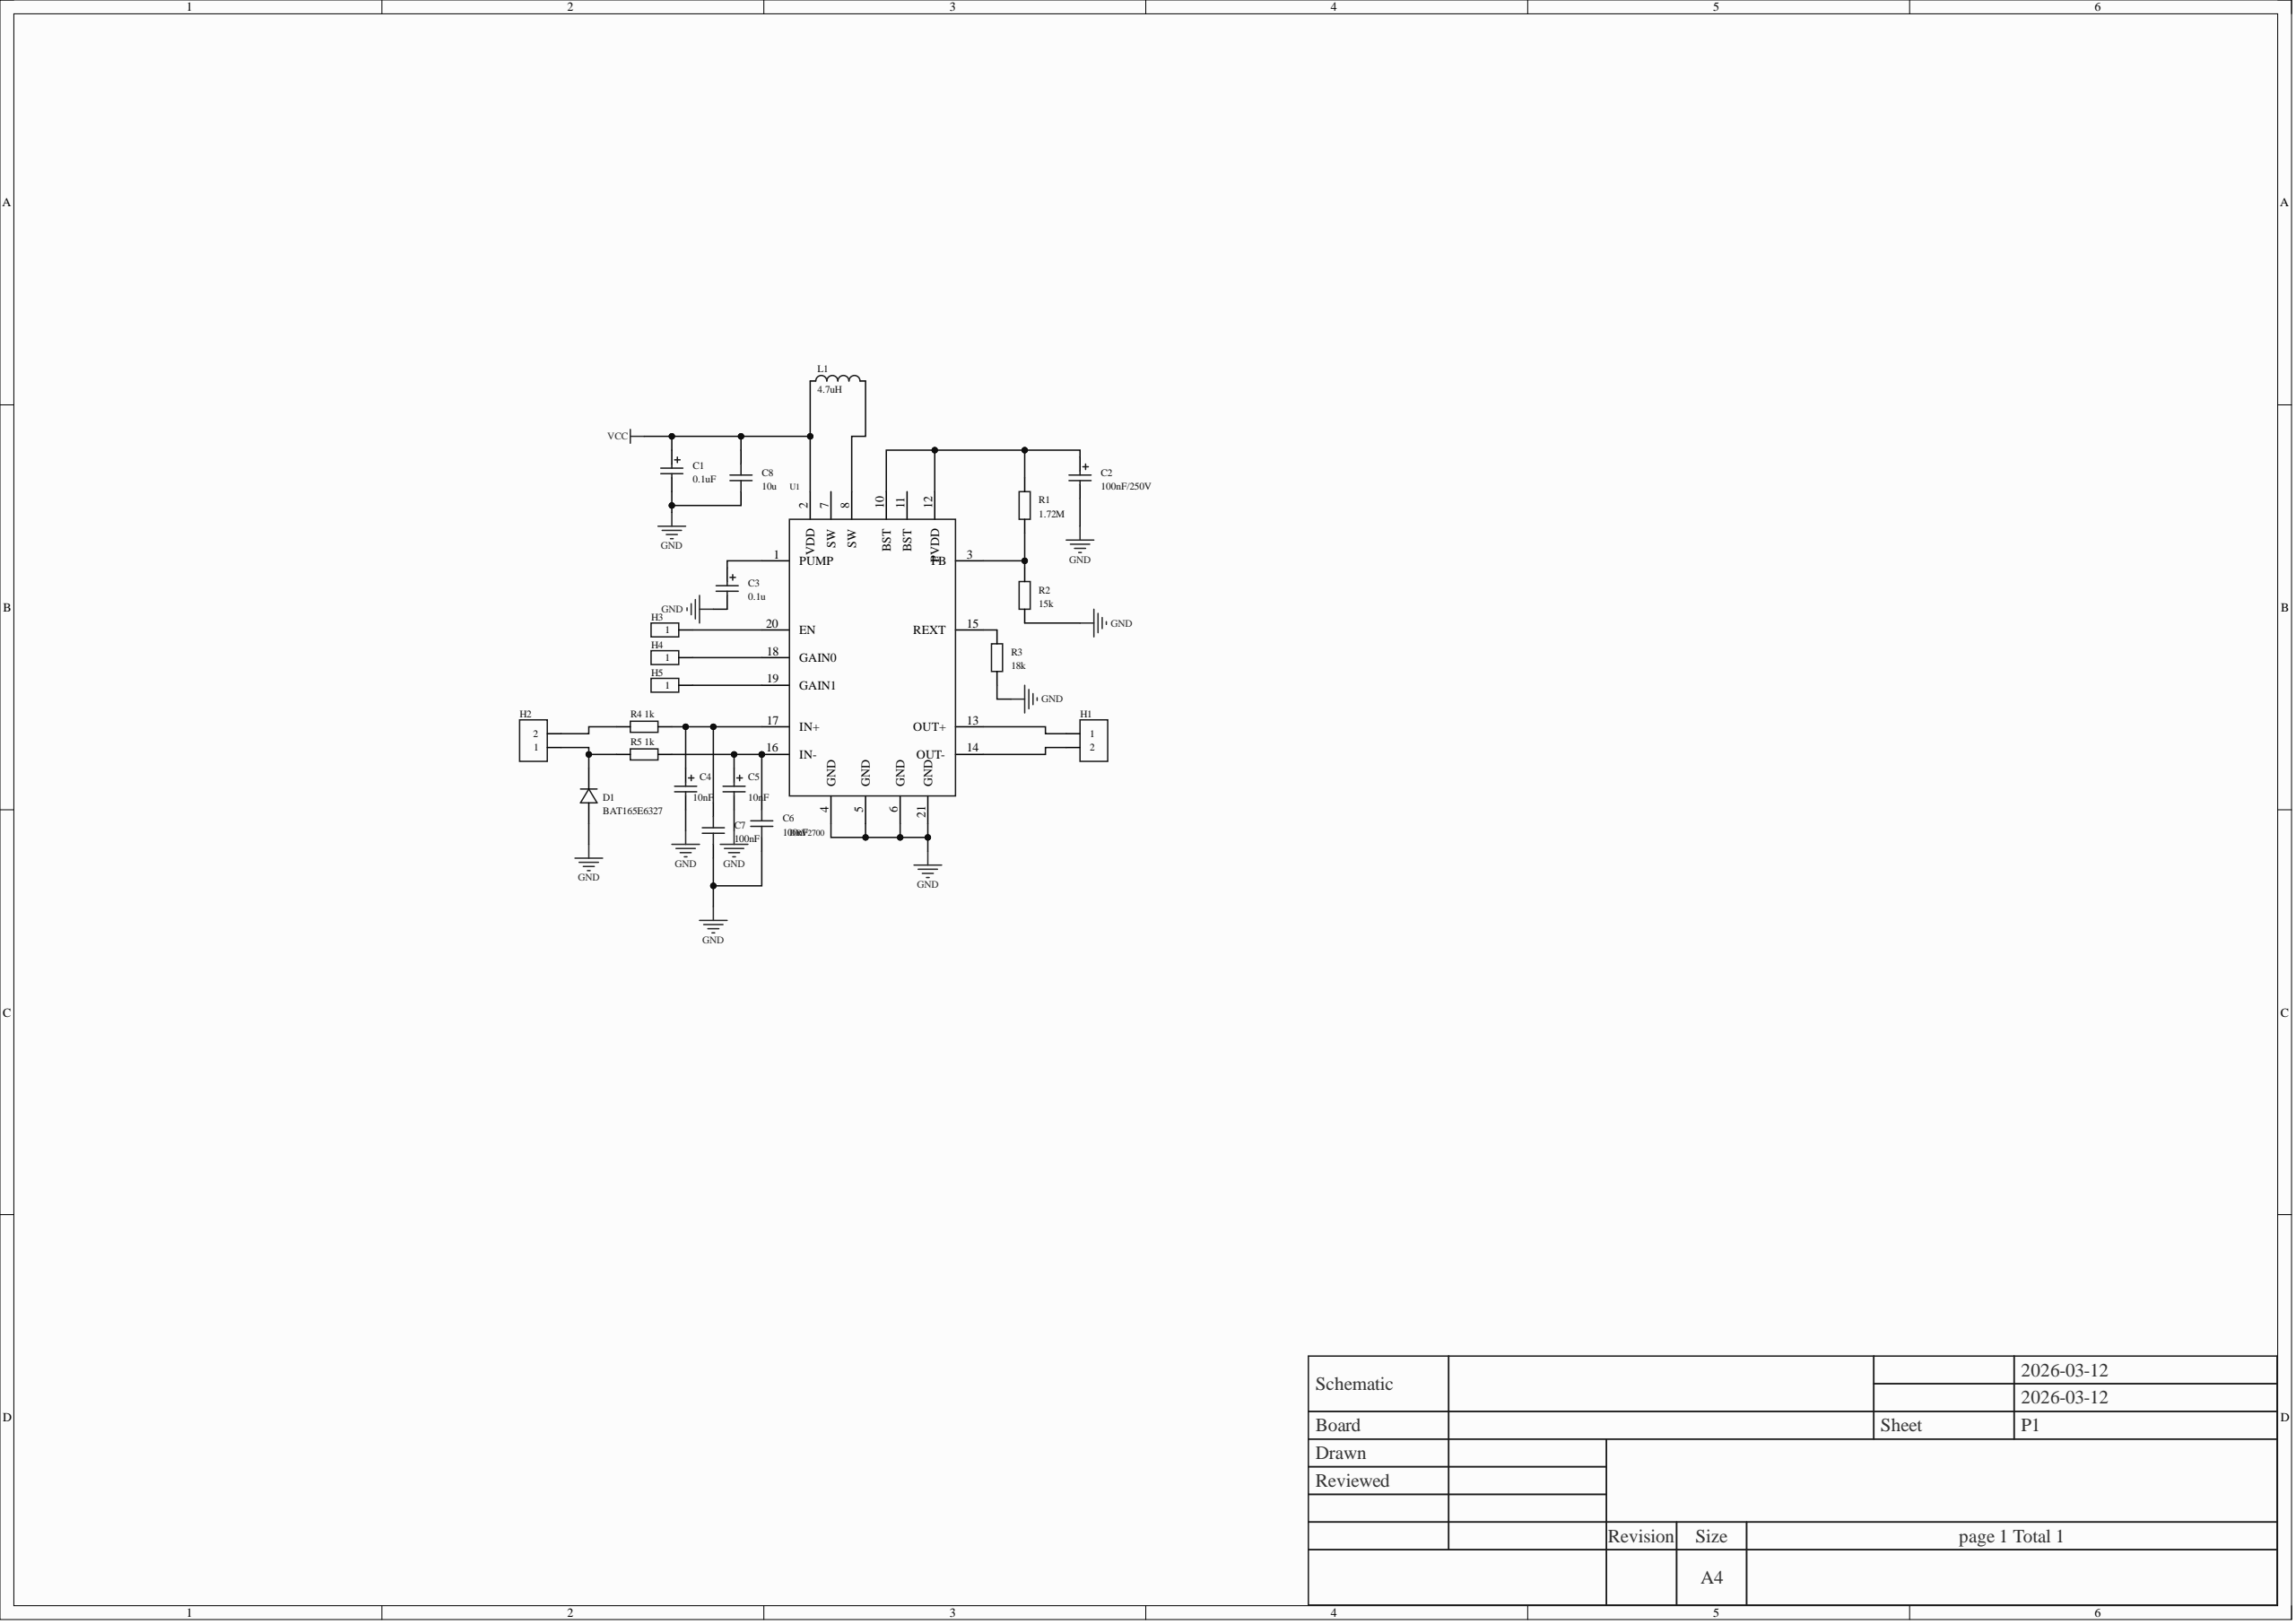Circuit board | Altium Designer | 21 parts | 16 nets
Bill of materials:
Comment,Description,Designator,Footprint,LibRef,Quantity
"0.1uF","","C1","C_Ele_SMD_3x5.4mm","C_Ele_SMD_3x5.4mm","1"
"100nF/250V","","C2","C_Ele_SMD_3x5.4mm","C_Ele_SMD_3x5.4mm","1"
"0.1u","","C3","C_Ele_SMD_3x5.4mm","C_Ele_SMD_3x5.4mm","1"
"10nF","","C4, C5","C_Ele_SMD_3x5.4mm","C_Ele_SMD_3x5.4mm","2"
"100nF","","C6, C7","C0805","CAP_0805","2"
"10u","","C8","C0805","CAP_0805","1"
"BAT165E6327","component BAT165E6327 compon Diode configuration: 1 independent; forward voltage (Vf): 740mV@750mA; DC reverse voltage (Vr): 40V; rectifier current: 750mA;","D1","SOD-323_L1.8-W1.3-LS2.5-RD","BAT165E6327","1"
"","","H1, H2","HDR-TH_2P-P2.54-V-F","HDR-F_2.54_1x2P","2"
"","","H3, H4, H5","HDR-TH_1P-V-M_XKB_X4611WV-01I-C28D40","HDR-M_2.54_1x1P","3"
"4.7uH","component SRG0420-4R7-M comp Inductance: 4.7uH; tolerance: ±20%; rated current: 3A; saturation current (Isat): 3.5A; type: molded inductor;","L1","IND-SMD_L4.6-W4.1-A","SRG0420-4R7-M","1"
"1.72M","","R1","Res_1W","Res_AXIAL-1W","1"
"15k","","R2","Res_1W","Res_AXIAL-1W","1"
"18k","","R3","Res_1/4W","Res_AXIAL-1W","1"
"1k","","R4, R5","Res_1/4W","Res_AXIAL-1W","2"
"DRV2700","","U1","TI-RGP20-2700X2700TP_V","DRV2700","1"
Netlist (Protel format):
[
C1
C_Ele_SMD_3x5.4mm
0.1uF



]
[
C2
C_Ele_SMD_3x5.4mm
100nF/250V



]
[
C3
C_Ele_SMD_3x5.4mm
0.1u



]
[
C4
C_Ele_SMD_3x5.4mm
10nF



]
[
C5
C_Ele_SMD_3x5.4mm
10nF



]
[
C6
C0805
100nF



]
[
C7
C0805
100nF



]
[
C8
C0805
10u



]
[
D1
SOD-323_L1.8-W1.3-LS2.5-RD
BAT165E6327



]
[
H1
HDR-TH_2P-P2.54-V-F




]
[
H2
HDR-TH_2P-P2.54-V-F




]
[
H3
HDR-TH_1P-V-M_XKB_X4611WV-01I-C28D40




]
[
H4
HDR-TH_1P-V-M_XKB_X4611WV-01I-C28D40




]
[
H5
HDR-TH_1P-V-M_XKB_X4611WV-01I-C28D40




]
[
L1
IND-SMD_L4.6-W4.1-A
4.7uH



]
[
R1
Res_1W
1.72M



]
[
R2
Res_1W
15k



]
[
R3
Res_1/4W
18k



]
[
R4
Res_1/4W
1k



]
[
R5
Res_1/4W
1k



]
[
U1
TI-RGP20-2700X2700TP_V
DRV2700



]
(
VCC
C1-1
C8-2
L1-1
U1-2
)
(
NetR3_2
R3-2
U1-15
)
(
NetR1_1
R1-1
R2-2
U1-3
)
(
NetL1_2
L1-2
U1-8
)
(
NetH5_1
H5-1
U1-19
)
(
NetH4_1
H4-1
U1-18
)
(
NetH3_1
H3-1
U1-20
)
(
NetH2_2
H2-2
R4-1
)
(
NetH1_2
H1-2
U1-14
)
(
NetH1_1
H1-1
U1-13
)
(
NetD1_1
D1-1
H2-1
R5-1
)
(
NetC5_1
C5-1
C6-2
R5-2
U1-16
)
(
NetC4_1
C4-1
C7-2
R4-2
U1-17
)
(
NetC3_1
C3-1
U1-1
)
(
NetC2_1
C2-1
R1-2
U1-10
U1-12
)
(
GND
C1-2
C2-2
C3-2
C4-2
C5-2
C6-1
C7-1
C8-1
D1-2
R2-1
R3-1
U1-4
U1-5
U1-6
U1-21
)